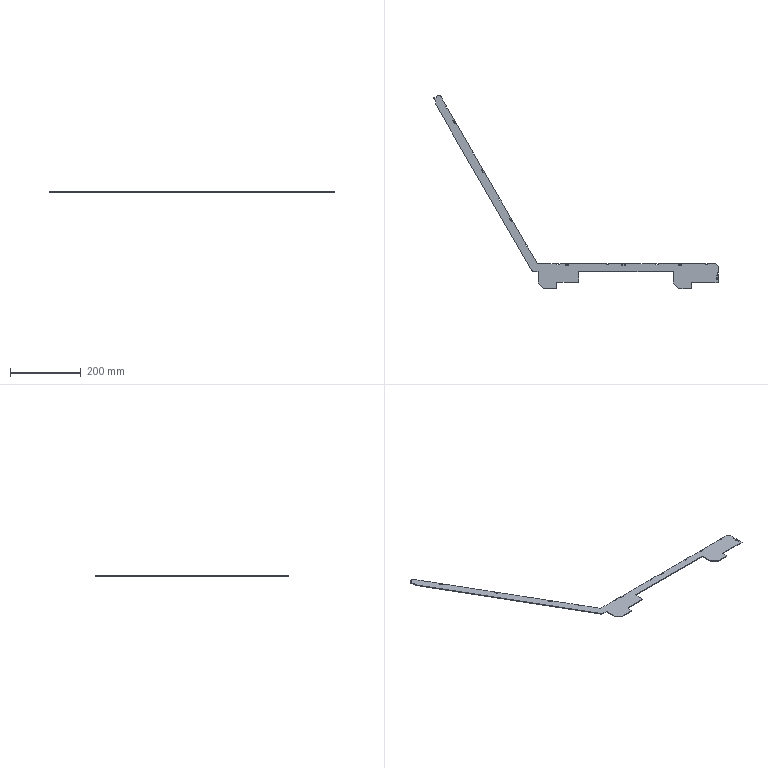Part | STEP file | zh004-1 | 1 solid | 96 faces | box 804.508 x 546.826 x 2 mm | volume 67085 mm3 | plane 92 | cylinder 4 | commonest cylinder face diameters 20 x2 4 x1 16 x1